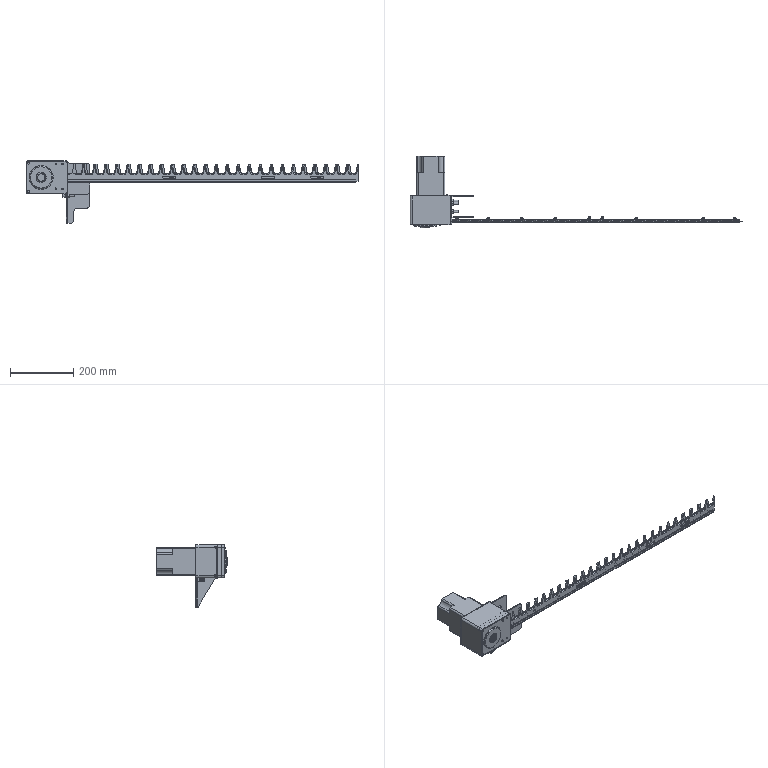Part | SolidWorks | 70 solids | 2414 faces | box 1053 x 226 x 197.5 mm | volume 1659148 mm3 | plane 1079 | cylinder 648 | cone 348 | torus 210 | sphere 110 | spline 19 | commonest cylinder face diameters 0.4 x74 10 x61 8 x44 18 x38 0.6 x36 5 x31